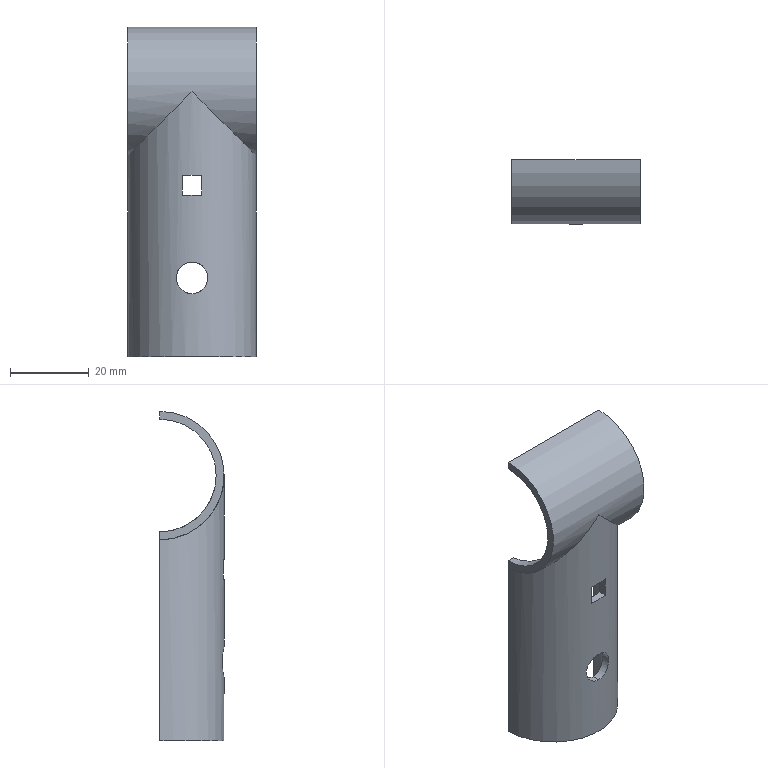Part | STEP file | F-D | 1 solid | 16 faces | box 32.6 x 16.3 x 83.6 mm | volume 7578 mm3 | plane 10 | cylinder 6 | commonest cylinder face diameters 8 x2 28.6 x2 32.6 x2
STEP:
#1=CARTESIAN_POINT('',(0.,48.7,-51.3));
#2=VERTEX_POINT('',#1);
#3=CARTESIAN_POINT('',(0.,48.7,-43.3));
#4=VERTEX_POINT('',#3);
#5=CARTESIAN_POINT('',(0.,48.7,-51.3));
#6=CARTESIAN_POINT('',(0.2485,48.7,-51.3));
#7=CARTESIAN_POINT('',(0.504,48.706,-51.277));
#8=CARTESIAN_POINT('',(0.8903,48.724,-51.202));
#9=CARTESIAN_POINT('',(1.02,48.732,-51.17));
#10=CARTESIAN_POINT('',(1.213,48.745,-51.112));
#11=CARTESIAN_POINT('',(1.31,48.753,-51.081));
#12=CARTESIAN_POINT('',(1.422,48.762,-51.039));
#13=CARTESIAN_POINT('',(1.478,48.767,-51.017));
#14=CARTESIAN_POINT('',(1.502,48.769,-51.007));
#15=CARTESIAN_POINT('',(1.518,48.771,-51.001));
#16=CARTESIAN_POINT('',(1.527,48.772,-50.997));
#17=CARTESIAN_POINT('',(1.643,48.783,-50.949));
#18=CARTESIAN_POINT('',(1.757,48.795,-50.896));
#19=CARTESIAN_POINT('',(1.932,48.815,-50.803));
#20=CARTESIAN_POINT('',(1.992,48.822,-50.769));
#21=CARTESIAN_POINT('',(2.082,48.834,-50.716));
#22=CARTESIAN_POINT('',(2.127,48.839,-50.688));
#23=CARTESIAN_POINT('',(2.18,48.847,-50.654));
#24=CARTESIAN_POINT('',(2.207,48.85,-50.636));
#25=CARTESIAN_POINT('',(2.218,48.852,-50.628));
#26=CARTESIAN_POINT('',(2.226,48.853,-50.623));
#27=CARTESIAN_POINT('',(2.231,48.854,-50.62));
#28=CARTESIAN_POINT('',(2.31,48.864,-50.567));
#29=CARTESIAN_POINT('',(2.4,48.878,-50.503));
#30=CARTESIAN_POINT('',(2.551,48.901,-50.382));
#31=CARTESIAN_POINT('',(2.604,48.909,-50.338));
#32=CARTESIAN_POINT('',(2.686,48.923,-50.264));
#33=CARTESIAN_POINT('',(2.714,48.928,-50.239));
#34=CARTESIAN_POINT('',(2.771,48.937,-50.185));
#35=CARTESIAN_POINT('',(2.798,48.942,-50.159));
#36=CARTESIAN_POINT('',(2.951,48.969,-50.006));
#37=CARTESIAN_POINT('',(3.05,48.987,-49.892));
#38=CARTESIAN_POINT('',(3.17,49.011,-49.741));
#39=CARTESIAN_POINT('',(3.205,49.018,-49.694));
#40=CARTESIAN_POINT('',(3.252,49.028,-49.629));
#41=CARTESIAN_POINT('',(3.274,49.032,-49.598));
#42=CARTESIAN_POINT('',(3.297,49.037,-49.565));
#43=CARTESIAN_POINT('',(3.308,49.039,-49.549));
#44=CARTESIAN_POINT('',(3.312,49.04,-49.542));
#45=CARTESIAN_POINT('',(3.315,49.041,-49.538));
#46=CARTESIAN_POINT('',(3.316,49.041,-49.537));
#47=CARTESIAN_POINT('',(3.401,49.058,-49.411));
#48=CARTESIAN_POINT('',(3.473,49.074,-49.29));
#49=CARTESIAN_POINT('',(3.566,49.095,-49.114));
#50=CARTESIAN_POINT('',(3.594,49.101,-49.056));
#51=CARTESIAN_POINT('',(3.634,49.11,-48.971));
#52=CARTESIAN_POINT('',(3.653,49.115,-48.929));
#53=CARTESIAN_POINT('',(3.674,49.12,-48.881));
#54=CARTESIAN_POINT('',(3.683,49.122,-48.861));
#55=CARTESIAN_POINT('',(3.689,49.123,-48.847));
#56=CARTESIAN_POINT('',(3.691,49.123,-48.842));
#57=CARTESIAN_POINT('',(3.907,49.174,-48.321));
#58=CARTESIAN_POINT('',(4.,49.198,-47.794));
#59=CARTESIAN_POINT('',(4.,49.198,-47.053));
#60=CARTESIAN_POINT('',(3.977,49.192,-46.798));
#61=CARTESIAN_POINT('',(3.902,49.174,-46.412));
#62=CARTESIAN_POINT('',(3.871,49.166,-46.282));
#63=CARTESIAN_POINT('',(3.813,49.152,-46.088));
#64=CARTESIAN_POINT('',(3.781,49.144,-45.991));
#65=CARTESIAN_POINT('',(3.739,49.135,-45.879));
#66=CARTESIAN_POINT('',(3.717,49.13,-45.823));
#67=CARTESIAN_POINT('',(3.708,49.127,-45.799));
#68=CARTESIAN_POINT('',(3.701,49.126,-45.783));
#69=CARTESIAN_POINT('',(3.697,49.125,-45.773));
#70=CARTESIAN_POINT('',(3.649,49.114,-45.658));
#71=CARTESIAN_POINT('',(3.597,49.102,-45.545));
#72=CARTESIAN_POINT('',(3.504,49.081,-45.369));
#73=CARTESIAN_POINT('',(3.47,49.074,-45.309));
#74=CARTESIAN_POINT('',(3.416,49.062,-45.219));
#75=CARTESIAN_POINT('',(3.388,49.056,-45.174));
#76=CARTESIAN_POINT('',(3.354,49.049,-45.12));
#77=CARTESIAN_POINT('',(3.336,49.045,-45.093));
#78=CARTESIAN_POINT('',(3.329,49.043,-45.082));
#79=CARTESIAN_POINT('',(3.324,49.042,-45.074));
#80=CARTESIAN_POINT('',(3.32,49.042,-45.069));
#81=CARTESIAN_POINT('',(3.271,49.032,-44.997));
#82=CARTESIAN_POINT('',(3.21,49.019,-44.91));
#83=CARTESIAN_POINT('',(3.09,48.995,-44.759));
#84=CARTESIAN_POINT('',(3.045,48.987,-44.705));
#85=CARTESIAN_POINT('',(2.97,48.973,-44.62));
#86=CARTESIAN_POINT('',(2.944,48.968,-44.591));
#87=CARTESIAN_POINT('',(2.888,48.958,-44.532));
#88=CARTESIAN_POINT('',(2.858,48.952,-44.501));
#89=CARTESIAN_POINT('',(2.712,48.927,-44.355));
#90=CARTESIAN_POINT('',(2.601,48.909,-44.258));
#91=CARTESIAN_POINT('',(2.45,48.885,-44.138));
#92=CARTESIAN_POINT('',(2.403,48.878,-44.102));
#93=CARTESIAN_POINT('',(2.336,48.868,-44.053));
#94=CARTESIAN_POINT('',(2.303,48.864,-44.03));
#95=CARTESIAN_POINT('',(2.268,48.859,-44.005));
#96=CARTESIAN_POINT('',(2.251,48.856,-43.993));
#97=CARTESIAN_POINT('',(2.243,48.855,-43.988));
#98=CARTESIAN_POINT('',(2.238,48.855,-43.985));
#99=CARTESIAN_POINT('',(2.237,48.854,-43.984));
#100=CARTESIAN_POINT('',(2.112,48.837,-43.9));
#101=CARTESIAN_POINT('',(1.991,48.822,-43.828));
#102=CARTESIAN_POINT('',(1.815,48.801,-43.735));
#103=CARTESIAN_POINT('',(1.758,48.795,-43.706));
#104=CARTESIAN_POINT('',(1.672,48.786,-43.666));
#105=CARTESIAN_POINT('',(1.63,48.782,-43.647));
#106=CARTESIAN_POINT('',(1.582,48.777,-43.626));
#107=CARTESIAN_POINT('',(1.561,48.775,-43.617));
#108=CARTESIAN_POINT('',(1.547,48.774,-43.611));
#109=CARTESIAN_POINT('',(1.542,48.773,-43.609));
#110=CARTESIAN_POINT('',(1.024,48.724,-43.394));
#111=CARTESIAN_POINT('',(0.497,48.7,-43.3));
#112=CARTESIAN_POINT('',(0.,48.7,-43.3));
#113=B_SPLINE_CURVE_WITH_KNOTS('',3,(#5,#6,#7,#8,#9,#10,#11,#12,#13,#14,#15,#16,#17,#18,#19,#20,#21,#22,#23,#24,#25,#26,#27,#28,#29,#30,#31,#32,#33,#34,#35,#36,#37,#38,#39,#40,#41,#42,#43,#44,#45,#46,#47,#48,#49,#50,#51,#52,#53,#54,#55,#56,#57,#58,#59,#60,#61,#62,#63,#64,#65,#66,#67,#68,#69,#70,#71,#72,#73,#74,#75,#76,#77,#78,#79,#80,#81,#82,#83,#84,#85,#86,#87,#88,#89,#90,#91,#92,#93,#94,#95,#96,#97,#98,#99,#100,#101,#102,#103,#104,#105,#106,#107,#108,#109,#110,#111,#112),.UNSPECIFIED.,.F.,.F.,(4,2,2,1,1,1,2,2,2,2,1,1,1,2,2,2,2,2,2,2,2,1,1,1,2,2,2,2,1,1,2,2,2,2,2,1,1,1,2,2,2,2,1,1,1,2,2,2,2,2,2,2,2,1,1,1,2,2,2,2,1,1,2,2,4),(0.5,0.5312,0.5469,0.5547,0.5586,0.5605,0.5615,0.5625,0.5781,0.5859,0.5898,0.5918,0.5928,0.5933,0.5937,0.6094,0.6172,0.6211,0.625,0.6406,0.6484,0.6523,0.6543,0.6553,0.6558,0.6562,0.6719,0.6797,0.6836,0.6855,0.6865,0.6875,0.75,0.7812,0.7969,0.8047,0.8086,0.8105,0.8115,0.8125,0.8281,0.8359,0.8398,0.8418,0.8428,0.8433,0.8437,0.8594,0.8672,0.8711,0.875,0.8906,0.8984,0.9023,0.9043,0.9053,0.9058,0.9062,0.9219,0.9297,0.9336,0.9355,0.9365,0.9375,1.),.UNSPECIFIED.);
#114=EDGE_CURVE('',#2,#4,#113,.T.);
#115=ORIENTED_EDGE('',*,*,#114,.T.);
#116=CARTESIAN_POINT('',(0.,50.7,-43.3));
#117=VERTEX_POINT('',#116);
#118=CARTESIAN_POINT('',(0.,130.,-43.3));
#119=DIRECTION('',(0.,1.,0.));
#120=VECTOR('',#119,1000.);
#121=LINE('',#118,#120);
#122=EDGE_CURVE('',#4,#117,#121,.T.);
#123=ORIENTED_EDGE('',*,*,#122,.T.);
#124=CARTESIAN_POINT('',(0.,50.7,-51.3));
#125=VERTEX_POINT('',#124);
#126=CARTESIAN_POINT('',(0.,50.7,-51.3));
#127=CARTESIAN_POINT('',(0.2655,50.7,-51.3));
#128=CARTESIAN_POINT('',(0.5263,50.707,-51.274));
#129=CARTESIAN_POINT('',(1.038,50.735,-51.172));
#130=CARTESIAN_POINT('',(1.29,50.756,-51.095));
#131=CARTESIAN_POINT('',(1.779,50.809,-50.892));
#132=CARTESIAN_POINT('',(2.009,50.84,-50.769));
#133=CARTESIAN_POINT('',(2.44,50.908,-50.481));
#134=CARTESIAN_POINT('',(2.641,50.945,-50.316));
#135=CARTESIAN_POINT('',(3.017,51.02,-49.94));
#136=CARTESIAN_POINT('',(3.182,51.058,-49.739));
#137=CARTESIAN_POINT('',(3.398,51.11,-49.415));
#138=CARTESIAN_POINT('',(3.465,51.126,-49.304));
#139=CARTESIAN_POINT('',(3.588,51.157,-49.074));
#140=CARTESIAN_POINT('',(3.643,51.172,-48.957));
#141=CARTESIAN_POINT('',(3.899,51.24,-48.342));
#142=CARTESIAN_POINT('',(4.,51.271,-47.83));
#143=CARTESIAN_POINT('',(4.,51.271,-47.035));
#144=CARTESIAN_POINT('',(3.975,51.263,-46.775));
#145=CARTESIAN_POINT('',(3.898,51.242,-46.391));
#146=CARTESIAN_POINT('',(3.866,51.233,-46.264));
#147=CARTESIAN_POINT('',(3.79,51.211,-46.013));
#148=CARTESIAN_POINT('',(3.745,51.199,-45.887));
#149=CARTESIAN_POINT('',(3.593,51.158,-45.522));
#150=CARTESIAN_POINT('',(3.471,51.127,-45.293));
#151=CARTESIAN_POINT('',(3.182,51.058,-44.862));
#152=CARTESIAN_POINT('',(3.016,51.02,-44.659));
#153=CARTESIAN_POINT('',(2.642,50.945,-44.285));
#154=CARTESIAN_POINT('',(2.44,50.908,-44.119));
#155=CARTESIAN_POINT('',(2.009,50.84,-43.831));
#156=CARTESIAN_POINT('',(1.78,50.809,-43.708));
#157=CARTESIAN_POINT('',(1.043,50.73,-43.402));
#158=CARTESIAN_POINT('',(0.5311,50.7,-43.3));
#159=CARTESIAN_POINT('',(0.,50.7,-43.3));
#160=B_SPLINE_CURVE_WITH_KNOTS('',3,(#126,#127,#128,#129,#130,#131,#132,#133,#134,#135,#136,#137,#138,#139,#140,#141,#142,#143,#144,#145,#146,#147,#148,#149,#150,#151,#152,#153,#154,#155,#156,#157,#158,#159),.UNSPECIFIED.,.F.,.F.,(4,2,2,2,2,2,2,2,2,2,2,2,2,2,2,2,4),(0.,0.0625,0.125,0.1875,0.25,0.3125,0.3438,0.375,0.5,0.5625,0.5938,0.625,0.6875,0.75,0.8125,0.875,1.),.UNSPECIFIED.);
#161=EDGE_CURVE('',#125,#117,#160,.T.);
#162=ORIENTED_EDGE('',*,*,#161,.F.);
#163=CARTESIAN_POINT('',(0.,130.,-51.3));
#164=DIRECTION('',(0.,1.,0.));
#165=VECTOR('',#164,1000.);
#166=LINE('',#163,#165);
#167=EDGE_CURVE('',#2,#125,#166,.T.);
#168=ORIENTED_EDGE('',*,*,#167,.F.);
#169=EDGE_LOOP('',(#115,#123,#162,#168));
#170=FACE_OUTER_BOUND('',#169,.T.);
#171=CARTESIAN_POINT('',(0.,130.,-47.3));
#172=DIRECTION('',(0.,1.,0.));
#173=DIRECTION('',(0.,0.,-1.));
#174=AXIS2_PLACEMENT_3D('',#171,#172,#173);
#175=CYLINDRICAL_SURFACE('',#174,4.);
#176=ADVANCED_FACE('',(#170),#175,.F.);
#177=CARTESIAN_POINT('',(16.3,65.,-16.3));
#178=VERTEX_POINT('',#177);
#179=CARTESIAN_POINT('',(16.3,65.,16.3));
#180=VERTEX_POINT('',#179);
#181=CARTESIAN_POINT('',(16.3,65.,0.));
#182=DIRECTION('',(-1.,0.,0.));
#183=DIRECTION('',(0.,0.,1.));
#184=AXIS2_PLACEMENT_3D('',#181,#182,#183);
#185=CIRCLE('',#184,16.3);
#186=EDGE_CURVE('',#178,#180,#185,.T.);
#187=ORIENTED_EDGE('',*,*,#186,.T.);
#188=CARTESIAN_POINT('',(-16.3,65.,16.3));
#189=VERTEX_POINT('',#188);
#190=CARTESIAN_POINT('',(16.3,65.,16.3));
#191=DIRECTION('',(1.,0.,0.));
#192=VECTOR('',#191,1000.);
#193=LINE('',#190,#192);
#194=EDGE_CURVE('',#189,#180,#193,.T.);
#195=ORIENTED_EDGE('',*,*,#194,.F.);
#196=CARTESIAN_POINT('',(-16.3,65.,-16.3));
#197=VERTEX_POINT('',#196);
#198=CARTESIAN_POINT('',(-16.3,65.,0.));
#199=DIRECTION('',(1.,0.,0.));
#200=DIRECTION('',(0.,1.,0.));
#201=AXIS2_PLACEMENT_3D('',#198,#199,#200);
#202=CIRCLE('',#201,16.3);
#203=EDGE_CURVE('',#189,#197,#202,.T.);
#204=ORIENTED_EDGE('',*,*,#203,.T.);
#205=CARTESIAN_POINT('',(0.,48.7,0.));
#206=VERTEX_POINT('',#205);
#207=CARTESIAN_POINT('',(0.,48.7,0.));
#208=CARTESIAN_POINT('',(-9.548,48.7,-9.548));
#209=CARTESIAN_POINT('',(-16.3,55.452,-16.3));
#210=CARTESIAN_POINT('',(-16.3,65.,-16.3));
#211=(BOUNDED_CURVE()B_SPLINE_CURVE(3,(#207,#208,#209,#210),.UNSPECIFIED.,.F.,.F.)B_SPLINE_CURVE_WITH_KNOTS((4,4),(4.712,6.283),.UNSPECIFIED.)CURVE()GEOMETRIC_REPRESENTATION_ITEM()RATIONAL_B_SPLINE_CURVE((1.,0.8047,0.8047,1.))REPRESENTATION_ITEM(''));
#212=EDGE_CURVE('',#206,#197,#211,.T.);
#213=ORIENTED_EDGE('',*,*,#212,.F.);
#214=CARTESIAN_POINT('',(16.3,65.,-16.3));
#215=CARTESIAN_POINT('',(16.3,55.452,-16.3));
#216=CARTESIAN_POINT('',(9.548,48.7,-9.548));
#217=CARTESIAN_POINT('',(0.,48.7,0.));
#218=(BOUNDED_CURVE()B_SPLINE_CURVE(3,(#214,#215,#216,#217),.UNSPECIFIED.,.F.,.F.)B_SPLINE_CURVE_WITH_KNOTS((4,4),(3.142,4.712),.UNSPECIFIED.)CURVE()GEOMETRIC_REPRESENTATION_ITEM()RATIONAL_B_SPLINE_CURVE((1.,0.8047,0.8047,1.))REPRESENTATION_ITEM(''));
#219=EDGE_CURVE('',#178,#206,#218,.T.);
#220=ORIENTED_EDGE('',*,*,#219,.F.);
#221=EDGE_LOOP('',(#187,#195,#204,#213,#220));
#222=FACE_OUTER_BOUND('',#221,.T.);
#223=CARTESIAN_POINT('',(16.3,65.,0.));
#224=DIRECTION('',(1.,0.,0.));
#225=DIRECTION('',(0.,0.,1.));
#226=AXIS2_PLACEMENT_3D('',#223,#224,#225);
#227=CYLINDRICAL_SURFACE('',#226,16.3);
#228=ADVANCED_FACE('',(#222),#227,.T.);
#229=ORIENTED_EDGE('',*,*,#203,.F.);
#230=CARTESIAN_POINT('',(-16.3,65.,14.3));
#231=VERTEX_POINT('',#230);
#232=CARTESIAN_POINT('',(-16.3,65.,0.));
#233=DIRECTION('',(0.,0.,-1.));
#234=VECTOR('',#233,1000.);
#235=LINE('',#232,#234);
#236=EDGE_CURVE('',#189,#231,#235,.T.);
#237=ORIENTED_EDGE('',*,*,#236,.T.);
#238=CARTESIAN_POINT('',(-16.3,65.,-14.3));
#239=VERTEX_POINT('',#238);
#240=CARTESIAN_POINT('',(-16.3,65.,0.));
#241=DIRECTION('',(-1.,0.,0.));
#242=DIRECTION('',(0.,-1.,0.));
#243=AXIS2_PLACEMENT_3D('',#240,#241,#242);
#244=CIRCLE('',#243,14.3);
#245=EDGE_CURVE('',#239,#231,#244,.T.);
#246=ORIENTED_EDGE('',*,*,#245,.F.);
#247=CARTESIAN_POINT('',(-16.3,65.,-16.3));
#248=DIRECTION('',(0.,0.,1.));
#249=VECTOR('',#248,1000.);
#250=LINE('',#247,#249);
#251=EDGE_CURVE('',#197,#239,#250,.T.);
#252=ORIENTED_EDGE('',*,*,#251,.F.);
#253=EDGE_LOOP('',(#229,#237,#246,#252));
#254=FACE_OUTER_BOUND('',#253,.T.);
#255=CARTESIAN_POINT('',(-16.3,65.,0.));
#256=DIRECTION('',(-1.,0.,0.));
#257=DIRECTION('',(0.,0.,1.));
#258=AXIS2_PLACEMENT_3D('',#255,#256,#257);
#259=PLANE('',#258);
#260=ADVANCED_FACE('',(#254),#259,.T.);
#261=CARTESIAN_POINT('',(-14.3,65.,-14.3));
#262=VERTEX_POINT('',#261);
#263=CARTESIAN_POINT('',(16.3,65.,-14.3));
#264=DIRECTION('',(-1.,0.,0.));
#265=VECTOR('',#264,1000.);
#266=LINE('',#263,#265);
#267=EDGE_CURVE('',#262,#239,#266,.T.);
#268=ORIENTED_EDGE('',*,*,#267,.F.);
#269=CARTESIAN_POINT('',(-14.3,65.,-67.3));
#270=VERTEX_POINT('',#269);
#271=CARTESIAN_POINT('',(-14.3,65.,-76.464));
#272=DIRECTION('',(0.,0.,1.));
#273=VECTOR('',#272,1000.);
#274=LINE('',#271,#273);
#275=EDGE_CURVE('',#270,#262,#274,.T.);
#276=ORIENTED_EDGE('',*,*,#275,.F.);
#277=CARTESIAN_POINT('',(-16.3,65.,-67.3));
#278=VERTEX_POINT('',#277);
#279=CARTESIAN_POINT('',(-26.203,65.,-67.3));
#280=DIRECTION('',(1.,0.,0.));
#281=VECTOR('',#280,1000.);
#282=LINE('',#279,#281);
#283=EDGE_CURVE('',#278,#270,#282,.T.);
#284=ORIENTED_EDGE('',*,*,#283,.F.);
#285=CARTESIAN_POINT('',(-16.3,65.,0.));
#286=DIRECTION('',(0.,0.,-1.));
#287=VECTOR('',#286,1000.);
#288=LINE('',#285,#287);
#289=EDGE_CURVE('',#197,#278,#288,.T.);
#290=ORIENTED_EDGE('',*,*,#289,.F.);
#291=ORIENTED_EDGE('',*,*,#251,.T.);
#292=EDGE_LOOP('',(#268,#276,#284,#290,#291));
#293=FACE_OUTER_BOUND('',#292,.T.);
#294=CARTESIAN_POINT('',(16.3,65.,-16.3));
#295=DIRECTION('',(0.,-1.,0.));
#296=DIRECTION('',(-1.,0.,0.));
#297=AXIS2_PLACEMENT_3D('',#294,#295,#296);
#298=PLANE('',#297);
#299=ADVANCED_FACE('',(#293),#298,.F.);
#300=ORIENTED_EDGE('',*,*,#114,.F.);
#301=CARTESIAN_POINT('',(0.,48.7,-43.3));
#302=CARTESIAN_POINT('',(-0.2485,48.7,-43.3));
#303=CARTESIAN_POINT('',(-0.504,48.706,-43.323));
#304=CARTESIAN_POINT('',(-0.8903,48.724,-43.398));
#305=CARTESIAN_POINT('',(-1.02,48.732,-43.43));
#306=CARTESIAN_POINT('',(-1.213,48.745,-43.488));
#307=CARTESIAN_POINT('',(-1.31,48.753,-43.519));
#308=CARTESIAN_POINT('',(-1.422,48.762,-43.561));
#309=CARTESIAN_POINT('',(-1.478,48.767,-43.583));
#310=CARTESIAN_POINT('',(-1.502,48.769,-43.593));
#311=CARTESIAN_POINT('',(-1.518,48.771,-43.599));
#312=CARTESIAN_POINT('',(-1.527,48.772,-43.603));
#313=CARTESIAN_POINT('',(-1.643,48.783,-43.651));
#314=CARTESIAN_POINT('',(-1.757,48.795,-43.704));
#315=CARTESIAN_POINT('',(-1.932,48.815,-43.797));
#316=CARTESIAN_POINT('',(-1.992,48.822,-43.831));
#317=CARTESIAN_POINT('',(-2.082,48.834,-43.884));
#318=CARTESIAN_POINT('',(-2.127,48.839,-43.912));
#319=CARTESIAN_POINT('',(-2.18,48.847,-43.946));
#320=CARTESIAN_POINT('',(-2.207,48.85,-43.964));
#321=CARTESIAN_POINT('',(-2.218,48.852,-43.972));
#322=CARTESIAN_POINT('',(-2.226,48.853,-43.977));
#323=CARTESIAN_POINT('',(-2.231,48.854,-43.98));
#324=CARTESIAN_POINT('',(-2.31,48.864,-44.033));
#325=CARTESIAN_POINT('',(-2.4,48.878,-44.097));
#326=CARTESIAN_POINT('',(-2.551,48.901,-44.218));
#327=CARTESIAN_POINT('',(-2.604,48.909,-44.262));
#328=CARTESIAN_POINT('',(-2.686,48.923,-44.336));
#329=CARTESIAN_POINT('',(-2.714,48.928,-44.361));
#330=CARTESIAN_POINT('',(-2.771,48.937,-44.415));
#331=CARTESIAN_POINT('',(-2.798,48.942,-44.441));
#332=CARTESIAN_POINT('',(-2.951,48.969,-44.594));
#333=CARTESIAN_POINT('',(-3.05,48.987,-44.708));
#334=CARTESIAN_POINT('',(-3.17,49.011,-44.859));
#335=CARTESIAN_POINT('',(-3.205,49.018,-44.906));
#336=CARTESIAN_POINT('',(-3.252,49.028,-44.971));
#337=CARTESIAN_POINT('',(-3.274,49.032,-45.002));
#338=CARTESIAN_POINT('',(-3.297,49.037,-45.035));
#339=CARTESIAN_POINT('',(-3.308,49.039,-45.051));
#340=CARTESIAN_POINT('',(-3.312,49.04,-45.058));
#341=CARTESIAN_POINT('',(-3.315,49.041,-45.062));
#342=CARTESIAN_POINT('',(-3.316,49.041,-45.063));
#343=CARTESIAN_POINT('',(-3.401,49.058,-45.189));
#344=CARTESIAN_POINT('',(-3.473,49.074,-45.31));
#345=CARTESIAN_POINT('',(-3.566,49.095,-45.486));
#346=CARTESIAN_POINT('',(-3.594,49.101,-45.544));
#347=CARTESIAN_POINT('',(-3.634,49.11,-45.629));
#348=CARTESIAN_POINT('',(-3.653,49.115,-45.671));
#349=CARTESIAN_POINT('',(-3.674,49.12,-45.719));
#350=CARTESIAN_POINT('',(-3.683,49.122,-45.739));
#351=CARTESIAN_POINT('',(-3.689,49.123,-45.753));
#352=CARTESIAN_POINT('',(-3.691,49.123,-45.758));
#353=CARTESIAN_POINT('',(-3.907,49.174,-46.279));
#354=CARTESIAN_POINT('',(-4.,49.198,-46.806));
#355=CARTESIAN_POINT('',(-4.,49.198,-47.547));
#356=CARTESIAN_POINT('',(-3.977,49.192,-47.802));
#357=CARTESIAN_POINT('',(-3.902,49.174,-48.188));
#358=CARTESIAN_POINT('',(-3.871,49.166,-48.318));
#359=CARTESIAN_POINT('',(-3.813,49.152,-48.512));
#360=CARTESIAN_POINT('',(-3.781,49.144,-48.609));
#361=CARTESIAN_POINT('',(-3.739,49.135,-48.721));
#362=CARTESIAN_POINT('',(-3.717,49.13,-48.777));
#363=CARTESIAN_POINT('',(-3.708,49.127,-48.801));
#364=CARTESIAN_POINT('',(-3.701,49.126,-48.817));
#365=CARTESIAN_POINT('',(-3.697,49.125,-48.827));
#366=CARTESIAN_POINT('',(-3.649,49.114,-48.942));
#367=CARTESIAN_POINT('',(-3.597,49.102,-49.055));
#368=CARTESIAN_POINT('',(-3.504,49.081,-49.231));
#369=CARTESIAN_POINT('',(-3.47,49.074,-49.291));
#370=CARTESIAN_POINT('',(-3.416,49.062,-49.381));
#371=CARTESIAN_POINT('',(-3.388,49.056,-49.426));
#372=CARTESIAN_POINT('',(-3.354,49.049,-49.48));
#373=CARTESIAN_POINT('',(-3.336,49.045,-49.507));
#374=CARTESIAN_POINT('',(-3.329,49.043,-49.518));
#375=CARTESIAN_POINT('',(-3.324,49.042,-49.526));
#376=CARTESIAN_POINT('',(-3.32,49.042,-49.531));
#377=CARTESIAN_POINT('',(-3.271,49.032,-49.603));
#378=CARTESIAN_POINT('',(-3.21,49.019,-49.69));
#379=CARTESIAN_POINT('',(-3.09,48.995,-49.841));
#380=CARTESIAN_POINT('',(-3.045,48.987,-49.895));
#381=CARTESIAN_POINT('',(-2.97,48.973,-49.98));
#382=CARTESIAN_POINT('',(-2.944,48.968,-50.009));
#383=CARTESIAN_POINT('',(-2.888,48.958,-50.068));
#384=CARTESIAN_POINT('',(-2.858,48.952,-50.099));
#385=CARTESIAN_POINT('',(-2.712,48.927,-50.245));
#386=CARTESIAN_POINT('',(-2.601,48.909,-50.342));
#387=CARTESIAN_POINT('',(-2.45,48.885,-50.462));
#388=CARTESIAN_POINT('',(-2.403,48.878,-50.498));
#389=CARTESIAN_POINT('',(-2.336,48.868,-50.547));
#390=CARTESIAN_POINT('',(-2.303,48.864,-50.57));
#391=CARTESIAN_POINT('',(-2.268,48.859,-50.595));
#392=CARTESIAN_POINT('',(-2.251,48.856,-50.607));
#393=CARTESIAN_POINT('',(-2.243,48.855,-50.612));
#394=CARTESIAN_POINT('',(-2.238,48.855,-50.615));
#395=CARTESIAN_POINT('',(-2.237,48.854,-50.616));
#396=CARTESIAN_POINT('',(-2.112,48.837,-50.7));
#397=CARTESIAN_POINT('',(-1.991,48.822,-50.772));
#398=CARTESIAN_POINT('',(-1.815,48.801,-50.865));
#399=CARTESIAN_POINT('',(-1.758,48.795,-50.894));
#400=CARTESIAN_POINT('',(-1.672,48.786,-50.934));
#401=CARTESIAN_POINT('',(-1.63,48.782,-50.953));
#402=CARTESIAN_POINT('',(-1.582,48.777,-50.974));
#403=CARTESIAN_POINT('',(-1.561,48.775,-50.983));
#404=CARTESIAN_POINT('',(-1.547,48.774,-50.989));
#405=CARTESIAN_POINT('',(-1.542,48.773,-50.991));
#406=CARTESIAN_POINT('',(-1.024,48.724,-51.206));
#407=CARTESIAN_POINT('',(-0.497,48.7,-51.3));
#408=CARTESIAN_POINT('',(0.,48.7,-51.3));
#409=B_SPLINE_CURVE_WITH_KNOTS('',3,(#301,#302,#303,#304,#305,#306,#307,#308,#309,#310,#311,#312,#313,#314,#315,#316,#317,#318,#319,#320,#321,#322,#323,#324,#325,#326,#327,#328,#329,#330,#331,#332,#333,#334,#335,#336,#337,#338,#339,#340,#341,#342,#343,#344,#345,#346,#347,#348,#349,#350,#351,#352,#353,#354,#355,#356,#357,#358,#359,#360,#361,#362,#363,#364,#365,#366,#367,#368,#369,#370,#371,#372,#373,#374,#375,#376,#377,#378,#379,#380,#381,#382,#383,#384,#385,#386,#387,#388,#389,#390,#391,#392,#393,#394,#395,#396,#397,#398,#399,#400,#401,#402,#403,#404,#405,#406,#407,#408),.UNSPECIFIED.,.F.,.F.,(4,2,2,1,1,1,2,2,2,2,1,1,1,2,2,2,2,2,2,2,2,1,1,1,2,2,2,2,1,1,2,2,2,2,2,1,1,1,2,2,2,2,1,1,1,2,2,2,2,2,2,2,2,1,1,1,2,2,2,2,1,1,2,2,4),(0.,0.03125,0.04687,0.05469,0.05859,0.06055,0.06152,0.0625,0.07812,0.08594,0.08984,0.0918,0.09277,0.09326,0.09375,0.1094,0.1172,0.1211,0.125,0.1406,0.1484,0.1523,0.1543,0.1553,0.1558,0.1562,0.1719,0.1797,0.1836,0.1855,0.1865,0.1875,0.25,0.2812,0.2969,0.3047,0.3086,0.3105,0.3115,0.3125,0.3281,0.3359,0.3398,0.3418,0.3428,0.3433,0.3437,0.3594,0.3672,0.3711,0.375,0.3906,0.3984,0.4023,0.4043,0.4053,0.4058,0.4062,0.4219,0.4297,0.4336,0.4355,0.4365,0.4375,0.5),.UNSPECIFIED.);
#410=EDGE_CURVE('',#4,#2,#409,.T.);
#411=ORIENTED_EDGE('',*,*,#410,.F.);
#412=EDGE_LOOP('',(#300,#411));
#413=FACE_BOUND('',#412,.T.);
#414=CARTESIAN_POINT('',(-2.5,48.893,-21.3));
#415=VERTEX_POINT('',#414);
#416=CARTESIAN_POINT('',(2.5,48.893,-21.3));
#417=VERTEX_POINT('',#416);
#418=CARTESIAN_POINT('',(0.,65.,-21.3));
#419=DIRECTION('',(0.,0.,1.));
#420=DIRECTION('',(1.,0.,0.));
#421=AXIS2_PLACEMENT_3D('',#418,#419,#420);
#422=CIRCLE('',#421,16.3);
#423=EDGE_CURVE('',#415,#417,#422,.T.);
#424=ORIENTED_EDGE('',*,*,#423,.T.);
#425=CARTESIAN_POINT('',(2.5,48.893,-26.3));
#426=VERTEX_POINT('',#425);
#427=CARTESIAN_POINT('',(2.5,48.893,-76.464));
#428=DIRECTION('',(0.,0.,-1.));
#429=VECTOR('',#428,1000.);
#430=LINE('',#427,#429);
#431=EDGE_CURVE('',#417,#426,#430,.T.);
#432=ORIENTED_EDGE('',*,*,#431,.T.);
#433=CARTESIAN_POINT('',(-2.5,48.893,-26.3));
#434=VERTEX_POINT('',#433);
#435=CARTESIAN_POINT('',(0.,65.,-26.3));
#436=DIRECTION('',(0.,0.,-1.));
#437=DIRECTION('',(-1.,0.,0.));
#438=AXIS2_PLACEMENT_3D('',#435,#436,#437);
#439=CIRCLE('',#438,16.3);
#440=EDGE_CURVE('',#426,#434,#439,.T.);
#441=ORIENTED_EDGE('',*,*,#440,.T.);
#442=CARTESIAN_POINT('',(-2.5,48.893,-76.464));
#443=DIRECTION('',(0.,0.,1.));
#444=VECTOR('',#443,1000.);
#445=LINE('',#442,#444);
#446=EDGE_CURVE('',#434,#415,#445,.T.);
#447=ORIENTED_EDGE('',*,*,#446,.T.);
#448=EDGE_LOOP('',(#424,#432,#441,#447));
#449=FACE_BOUND('',#448,.T.);
#450=CARTESIAN_POINT('',(16.3,65.,-67.3));
#451=VERTEX_POINT('',#450);
#452=CARTESIAN_POINT('',(16.3,65.,-76.464));
#453=DIRECTION('',(0.,0.,-1.));
#454=VECTOR('',#453,1000.);
#455=LINE('',#452,#454);
#456=EDGE_CURVE('',#178,#451,#455,.T.);
#457=ORIENTED_EDGE('',*,*,#456,.F.);
#458=ORIENTED_EDGE('',*,*,#219,.T.);
#459=ORIENTED_EDGE('',*,*,#212,.T.);
#460=ORIENTED_EDGE('',*,*,#289,.T.);
#461=CARTESIAN_POINT('',(0.,65.,-67.3));
#462=DIRECTION('',(0.,0.,-1.));
#463=DIRECTION('',(-1.,0.,0.));
#464=AXIS2_PLACEMENT_3D('',#461,#462,#463);
#465=CIRCLE('',#464,16.3);
#466=EDGE_CURVE('',#451,#278,#465,.T.);
#467=ORIENTED_EDGE('',*,*,#466,.F.);
#468=EDGE_LOOP('',(#457,#458,#459,#460,#467));
#469=FACE_OUTER_BOUND('',#468,.T.);
#470=CARTESIAN_POINT('',(0.,65.,-76.464));
#471=DIRECTION('',(0.,0.,-1.));
#472=DIRECTION('',(1.,0.,0.));
#473=AXIS2_PLACEMENT_3D('',#470,#471,#472);
#474=CYLINDRICAL_SURFACE('',#473,16.3);
#475=ADVANCED_FACE('',(#413,#449,#469),#474,.T.);
#476=ORIENTED_EDGE('',*,*,#161,.T.);
#477=CARTESIAN_POINT('',(0.,50.7,-43.3));
#478=CARTESIAN_POINT('',(-0.2655,50.7,-43.3));
#479=CARTESIAN_POINT('',(-0.5263,50.707,-43.326));
#480=CARTESIAN_POINT('',(-1.038,50.735,-43.428));
#481=CARTESIAN_POINT('',(-1.29,50.756,-43.505));
#482=CARTESIAN_POINT('',(-1.779,50.809,-43.708));
#483=CARTESIAN_POINT('',(-2.009,50.84,-43.831));
#484=CARTESIAN_POINT('',(-2.44,50.908,-44.119));
#485=CARTESIAN_POINT('',(-2.641,50.945,-44.284));
#486=CARTESIAN_POINT('',(-3.017,51.02,-44.66));
#487=CARTESIAN_POINT('',(-3.182,51.058,-44.861));
#488=CARTESIAN_POINT('',(-3.398,51.11,-45.185));
#489=CARTESIAN_POINT('',(-3.465,51.126,-45.296));
#490=CARTESIAN_POINT('',(-3.588,51.157,-45.526));
#491=CARTESIAN_POINT('',(-3.643,51.172,-45.643));
#492=CARTESIAN_POINT('',(-3.899,51.24,-46.258));
#493=CARTESIAN_POINT('',(-4.,51.271,-46.77));
#494=CARTESIAN_POINT('',(-4.,51.271,-47.565));
#495=CARTESIAN_POINT('',(-3.975,51.263,-47.825));
#496=CARTESIAN_POINT('',(-3.898,51.242,-48.209));
#497=CARTESIAN_POINT('',(-3.866,51.233,-48.336));
#498=CARTESIAN_POINT('',(-3.79,51.211,-48.587));
#499=CARTESIAN_POINT('',(-3.745,51.199,-48.713));
#500=CARTESIAN_POINT('',(-3.593,51.158,-49.078));
#501=CARTESIAN_POINT('',(-3.471,51.127,-49.307));
#502=CARTESIAN_POINT('',(-3.182,51.058,-49.738));
#503=CARTESIAN_POINT('',(-3.016,51.02,-49.941));
#504=CARTESIAN_POINT('',(-2.642,50.945,-50.315));
#505=CARTESIAN_POINT('',(-2.44,50.908,-50.481));
#506=CARTESIAN_POINT('',(-2.009,50.84,-50.769));
#507=CARTESIAN_POINT('',(-1.78,50.809,-50.892));
#508=CARTESIAN_POINT('',(-1.043,50.73,-51.198));
#509=CARTESIAN_POINT('',(-0.5311,50.7,-51.3));
#510=CARTESIAN_POINT('',(0.,50.7,-51.3));
#511=B_SPLINE_CURVE_WITH_KNOTS('',3,(#477,#478,#479,#480,#481,#482,#483,#484,#485,#486,#487,#488,#489,#490,#491,#492,#493,#494,#495,#496,#497,#498,#499,#500,#501,#502,#503,#504,#505,#506,#507,#508,#509,#510),.UNSPECIFIED.,.F.,.F.,(4,2,2,2,2,2,2,2,2,2,2,2,2,2,2,2,4),(0.,0.0625,0.125,0.1875,0.25,0.3125,0.3438,0.375,0.5,0.5625,0.5938,0.625,0.6875,0.75,0.8125,0.875,1.),.UNSPECIFIED.);
#512=EDGE_CURVE('',#117,#125,#511,.T.);
#513=ORIENTED_EDGE('',*,*,#512,.T.);
#514=EDGE_LOOP('',(#476,#513));
#515=FACE_BOUND('',#514,.T.);
#516=CARTESIAN_POINT('',(2.5,50.92,-21.3));
#517=VERTEX_POINT('',#516);
#518=CARTESIAN_POINT('',(2.5,50.92,-26.3));
#519=VERTEX_POINT('',#518);
#520=CARTESIAN_POINT('',(2.5,50.92,-76.464));
#521=DIRECTION('',(0.,0.,-1.));
#522=VECTOR('',#521,1000.);
#523=LINE('',#520,#522);
#524=EDGE_CURVE('',#517,#519,#523,.T.);
#525=ORIENTED_EDGE('',*,*,#524,.F.);
#526=CARTESIAN_POINT('',(-2.5,50.92,-21.3));
#527=VERTEX_POINT('',#526);
#528=CARTESIAN_POINT('',(0.,65.,-21.3));
#529=DIRECTION('',(0.,0.,1.));
#530=DIRECTION('',(1.,0.,0.));
#531=AXIS2_PLACEMENT_3D('',#528,#529,#530);
#532=CIRCLE('',#531,14.3);
#533=EDGE_CURVE('',#527,#517,#532,.T.);
#534=ORIENTED_EDGE('',*,*,#533,.F.);
#535=CARTESIAN_POINT('',(-2.5,50.92,-26.3));
#536=VERTEX_POINT('',#535);
#537=CARTESIAN_POINT('',(-2.5,50.92,-76.464));
#538=DIRECTION('',(0.,0.,1.));
#539=VECTOR('',#538,1000.);
#540=LINE('',#537,#539);
#541=EDGE_CURVE('',#536,#527,#540,.T.);
#542=ORIENTED_EDGE('',*,*,#541,.F.);
#543=CARTESIAN_POINT('',(0.,65.,-26.3));
#544=DIRECTION('',(0.,0.,-1.));
#545=DIRECTION('',(-1.,0.,0.));
#546=AXIS2_PLACEMENT_3D('',#543,#544,#545);
#547=CIRCLE('',#546,14.3);
#548=EDGE_CURVE('',#519,#536,#547,.T.);
#549=ORIENTED_EDGE('',*,*,#548,.F.);
#550=EDGE_LOOP('',(#525,#534,#542,#549));
#551=FACE_BOUND('',#550,.T.);
#552=CARTESIAN_POINT('',(14.3,65.,-67.3));
#553=VERTEX_POINT('',#552);
#554=CARTESIAN_POINT('',(0.,65.,-67.3));
#555=DIRECTION('',(0.,0.,-1.));
#556=DIRECTION('',(-1.,0.,0.));
#557=AXIS2_PLACEMENT_3D('',#554,#555,#556);
#558=CIRCLE('',#557,14.3);
#559=EDGE_CURVE('',#553,#270,#558,.T.);
#560=ORIENTED_EDGE('',*,*,#559,.T.);
#561=ORIENTED_EDGE('',*,*,#275,.T.);
#562=CARTESIAN_POINT('',(0.,50.7,0.));
#563=VERTEX_POINT('',#562);
#564=CARTESIAN_POINT('',(-14.3,65.,-14.3));
#565=CARTESIAN_POINT('',(-14.3,56.623,-14.3));
#566=CARTESIAN_POINT('',(-8.377,50.7,-8.377));
#567=CARTESIAN_POINT('',(0.,50.7,0.));
#568=(BOUNDED_CURVE()B_SPLINE_CURVE(3,(#564,#565,#566,#567),.UNSPECIFIED.,.F.,.F.)B_SPLINE_CURVE_WITH_KNOTS((4,4),(0.,1.571),.UNSPECIFIED.)CURVE()GEOMETRIC_REPRESENTATION_ITEM()RATIONAL_B_SPLINE_CURVE((1.,0.8047,0.8047,1.))REPRESENTATION_ITEM(''));
#569=EDGE_CURVE('',#262,#563,#568,.T.);
#570=ORIENTED_EDGE('',*,*,#569,.T.);
#571=CARTESIAN_POINT('',(14.3,65.,-14.3));
#572=VERTEX_POINT('',#571);
#573=CARTESIAN_POINT('',(0.,50.7,0.));
#574=CARTESIAN_POINT('',(8.377,50.7,-8.377));
#575=CARTESIAN_POINT('',(14.3,56.623,-14.3));
#576=CARTESIAN_POINT('',(14.3,65.,-14.3));
#577=(BOUNDED_CURVE()B_SPLINE_CURVE(3,(#573,#574,#575,#576),.UNSPECIFIED.,.F.,.F.)B_SPLINE_CURVE_WITH_KNOTS((4,4),(1.571,3.142),.UNSPECIFIED.)CURVE()GEOMETRIC_REPRESENTATION_ITEM()RATIONAL_B_SPLINE_CURVE((1.,0.8047,0.8047,1.))REPRESENTATION_ITEM(''));
#578=EDGE_CURVE('',#563,#572,#577,.T.);
#579=ORIENTED_EDGE('',*,*,#578,.T.);
#580=CARTESIAN_POINT('',(14.3,65.,-76.464));
#581=DIRECTION('',(0.,0.,-1.));
#582=VECTOR('',#581,1000.);
#583=LINE('',#580,#582);
#584=EDGE_CURVE('',#572,#553,#583,.T.);
#585=ORIENTED_EDGE('',*,*,#584,.T.);
#586=EDGE_LOOP('',(#560,#561,#570,#579,#585));
#587=FACE_OUTER_BOUND('',#586,.T.);
#588=CARTESIAN_POINT('',(0.,65.,-76.464));
#589=DIRECTION('',(0.,0.,-1.));
#590=DIRECTION('',(1.,0.,0.));
#591=AXIS2_PLACEMENT_3D('',#588,#589,#590);
#592=CYLINDRICAL_SURFACE('',#591,14.3);
#593=ADVANCED_FACE('',(#515,#551,#587),#592,.F.);
#594=ORIENTED_EDGE('',*,*,#466,.T.);
#595=ORIENTED_EDGE('',*,*,#283,.T.);
#596=ORIENTED_EDGE('',*,*,#559,.F.);
#597=CARTESIAN_POINT('',(-26.203,65.,-67.3));
#598=DIRECTION('',(1.,0.,0.));
#599=VECTOR('',#598,1000.);
#600=LINE('',#597,#599);
#601=EDGE_CURVE('',#553,#451,#600,.T.);
#602=ORIENTED_EDGE('',*,*,#601,.T.);
#603=EDGE_LOOP('',(#594,#595,#596,#602));
#604=FACE_OUTER_BOUND('',#603,.T.);
#605=CARTESIAN_POINT('',(-26.203,126.385,-67.3));
#606=DIRECTION('',(0.,0.,-1.));
#607=DIRECTION('',(0.,-1.,0.));
#608=AXIS2_PLACEMENT_3D('',#605,#606,#607);
#609=PLANE('',#608);
#610=ADVANCED_FACE('',(#604),#609,.T.);
#611=CARTESIAN_POINT('',(16.3,65.,14.3));
#612=VERTEX_POINT('',#611);
#613=CARTESIAN_POINT('',(16.3,65.,20.242));
#614=DIRECTION('',(0.,0.,-1.));
#615=VECTOR('',#614,1000.);
#616=LINE('',#613,#615);
#617=EDGE_CURVE('',#180,#612,#616,.T.);
#618=ORIENTED_EDGE('',*,*,#617,.T.);
#619=CARTESIAN_POINT('',(16.3,65.,14.3));
#620=DIRECTION('',(-1.,0.,0.));
#621=VECTOR('',#620,1000.);
#622=LINE('',#619,#621);
#623=EDGE_CURVE('',#612,#231,#622,.T.);
#624=ORIENTED_EDGE('',*,*,#623,.T.);
#625=ORIENTED_EDGE('',*,*,#236,.F.);
#626=ORIENTED_EDGE('',*,*,#194,.T.);
#627=EDGE_LOOP('',(#618,#624,#625,#626));
#628=FACE_OUTER_BOUND('',#627,.T.);
#629=CARTESIAN_POINT('',(64.481,65.,40.483));
#630=DIRECTION('',(0.,1.,0.));
#631=DIRECTION('',(1.,0.,0.));
#632=AXIS2_PLACEMENT_3D('',#629,#630,#631);
#633=PLANE('',#632);
#634=ADVANCED_FACE('',(#628),#633,.T.);
#635=ORIENTED_EDGE('',*,*,#524,.T.);
#636=CARTESIAN_POINT('',(2.5,127.576,-26.3));
#637=DIRECTION('',(0.,-1.,0.));
#638=VECTOR('',#637,1000.);
#639=LINE('',#636,#638);
#640=EDGE_CURVE('',#519,#426,#639,.T.);
#641=ORIENTED_EDGE('',*,*,#640,.T.);
#642=ORIENTED_EDGE('',*,*,#431,.F.);
#643=CARTESIAN_POINT('',(2.5,127.576,-21.3));
#644=DIRECTION('',(0.,-1.,0.));
#645=VECTOR('',#644,1000.);
#646=LINE('',#643,#645);
#647=EDGE_CURVE('',#517,#417,#646,.T.);
#648=ORIENTED_EDGE('',*,*,#647,.F.);
#649=EDGE_LOOP('',(#635,#641,#642,#648));
#650=FACE_OUTER_BOUND('',#649,.T.);
#651=CARTESIAN_POINT('',(2.5,127.576,-26.3));
#652=DIRECTION('',(1.,0.,0.));
#653=DIRECTION('',(0.,1.,0.));
#654=AXIS2_PLACEMENT_3D('',#651,#652,#653);
#655=PLANE('',#654);
#656=ADVANCED_FACE('',(#650),#655,.F.);
#657=ORIENTED_EDGE('',*,*,#533,.T.);
#658=ORIENTED_EDGE('',*,*,#647,.T.);
#659=ORIENTED_EDGE('',*,*,#423,.F.);
#660=CARTESIAN_POINT('',(-2.5,127.576,-21.3));
#661=DIRECTION('',(0.,-1.,0.));
#662=VECTOR('',#661,1000.);
#663=LINE('',#660,#662);
#664=EDGE_CURVE('',#527,#415,#663,.T.);
#665=ORIENTED_EDGE('',*,*,#664,.F.);
#666=EDGE_LOOP('',(#657,#658,#659,#665));
#667=FACE_OUTER_BOUND('',#666,.T.);
#668=CARTESIAN_POINT('',(2.5,127.576,-21.3));
#669=DIRECTION('',(0.,0.,1.));
#670=DIRECTION('',(1.,0.,0.));
#671=AXIS2_PLACEMENT_3D('',#668,#669,#670);
#672=PLANE('',#671);
#673=ADVANCED_FACE('',(#667),#672,.F.);
#674=ORIENTED_EDGE('',*,*,#541,.T.);
#675=ORIENTED_EDGE('',*,*,#664,.T.);
#676=ORIENTED_EDGE('',*,*,#446,.F.);
#677=CARTESIAN_POINT('',(-2.5,127.576,-26.3));
#678=DIRECTION('',(0.,-1.,0.));
#679=VECTOR('',#678,1000.);
#680=LINE('',#677,#679);
#681=EDGE_CURVE('',#536,#434,#680,.T.);
#682=ORIENTED_EDGE('',*,*,#681,.F.);
#683=EDGE_LOOP('',(#674,#675,#676,#682));
#684=FACE_OUTER_BOUND('',#683,.T.);
#685=CARTESIAN_POINT('',(-2.5,127.576,-21.3));
#686=DIRECTION('',(-1.,0.,0.));
#687=DIRECTION('',(0.,0.,1.));
#688=AXIS2_PLACEMENT_3D('',#685,#686,#687);
#689=PLANE('',#688);
#690=ADVANCED_FACE('',(#684),#689,.F.);
#691=ORIENTED_EDGE('',*,*,#548,.T.);
#692=ORIENTED_EDGE('',*,*,#681,.T.);
#693=ORIENTED_EDGE('',*,*,#440,.F.);
#694=ORIENTED_EDGE('',*,*,#640,.F.);
#695=EDGE_LOOP('',(#691,#692,#693,#694));
#696=FACE_OUTER_BOUND('',#695,.T.);
#697=CARTESIAN_POINT('',(-2.5,127.576,-26.3));
#698=DIRECTION('',(0.,0.,-1.));
#699=DIRECTION('',(0.,-1.,0.));
#700=AXIS2_PLACEMENT_3D('',#697,#698,#699);
#701=PLANE('',#700);
#702=ADVANCED_FACE('',(#696),#701,.F.);
#703=ORIENTED_EDGE('',*,*,#122,.F.);
#704=ORIENTED_EDGE('',*,*,#410,.T.);
#705=ORIENTED_EDGE('',*,*,#167,.T.);
#706=ORIENTED_EDGE('',*,*,#512,.F.);
#707=EDGE_LOOP('',(#703,#704,#705,#706));
#708=FACE_OUTER_BOUND('',#707,.T.);
#709=CARTESIAN_POINT('',(0.,130.,-47.3));
#710=DIRECTION('',(0.,1.,0.));
#711=DIRECTION('',(0.,0.,-1.));
#712=AXIS2_PLACEMENT_3D('',#709,#710,#711);
#713=CYLINDRICAL_SURFACE('',#712,4.);
#714=ADVANCED_FACE('',(#708),#713,.F.);
#715=CARTESIAN_POINT('',(16.3,65.,-14.3));
#716=VERTEX_POINT('',#715);
#717=CARTESIAN_POINT('',(16.3,65.,-8.15));
#718=DIRECTION('',(0.,0.,-1.));
#719=VECTOR('',#718,1000.);
#720=LINE('',#717,#719);
#721=EDGE_CURVE('',#716,#178,#720,.T.);
#722=ORIENTED_EDGE('',*,*,#721,.T.);
#723=ORIENTED_EDGE('',*,*,#456,.T.);
#724=ORIENTED_EDGE('',*,*,#601,.F.);
#725=ORIENTED_EDGE('',*,*,#584,.F.);
#726=CARTESIAN_POINT('',(16.3,65.,-14.3));
#727=DIRECTION('',(-1.,0.,0.));
#728=VECTOR('',#727,1000.);
#729=LINE('',#726,#728);
#730=EDGE_CURVE('',#716,#572,#729,.T.);
#731=ORIENTED_EDGE('',*,*,#730,.F.);
#732=EDGE_LOOP('',(#722,#723,#724,#725,#731));
#733=FACE_OUTER_BOUND('',#732,.T.);
#734=CARTESIAN_POINT('',(16.3,65.,-16.3));
#735=DIRECTION('',(0.,-1.,0.));
#736=DIRECTION('',(-1.,0.,0.));
#737=AXIS2_PLACEMENT_3D('',#734,#735,#736);
#738=PLANE('',#737);
#739=ADVANCED_FACE('',(#733),#738,.F.);
#740=CARTESIAN_POINT('',(16.3,65.,0.));
#741=DIRECTION('',(1.,0.,0.));
#742=DIRECTION('',(0.,0.,1.));
#743=AXIS2_PLACEMENT_3D('',#740,#741,#742);
#744=CIRCLE('',#743,14.3);
#745=EDGE_CURVE('',#612,#716,#744,.T.);
#746=ORIENTED_EDGE('',*,*,#745,.T.);
#747=ORIENTED_EDGE('',*,*,#730,.T.);
#748=ORIENTED_EDGE('',*,*,#578,.F.);
#749=ORIENTED_EDGE('',*,*,#569,.F.);
#750=ORIENTED_EDGE('',*,*,#267,.T.);
#751=ORIENTED_EDGE('',*,*,#245,.T.);
#752=ORIENTED_EDGE('',*,*,#623,.F.);
#753=EDGE_LOOP('',(#746,#747,#748,#749,#750,#751,#752));
#754=FACE_OUTER_BOUND('',#753,.T.);
#755=CARTESIAN_POINT('',(16.3,65.,0.));
#756=DIRECTION('',(1.,0.,0.));
#757=DIRECTION('',(0.,0.,1.));
#758=AXIS2_PLACEMENT_3D('',#755,#756,#757);
#759=CYLINDRICAL_SURFACE('',#758,14.3);
#760=ADVANCED_FACE('',(#754),#759,.F.);
#761=ORIENTED_EDGE('',*,*,#617,.F.);
#762=ORIENTED_EDGE('',*,*,#186,.F.);
#763=ORIENTED_EDGE('',*,*,#721,.F.);
#764=ORIENTED_EDGE('',*,*,#745,.F.);
#765=EDGE_LOOP('',(#761,#762,#763,#764));
#766=FACE_OUTER_BOUND('',#765,.T.);
#767=CARTESIAN_POINT('',(16.3,65.,0.));
#768=DIRECTION('',(-1.,0.,0.));
#769=DIRECTION('',(0.,0.,1.));
#770=AXIS2_PLACEMENT_3D('',#767,#768,#769);
#771=PLANE('',#770);
#772=ADVANCED_FACE('',(#766),#771,.F.);
#773=CLOSED_SHELL('',(#176,#228,#260,#299,#475,#593,#610,#634,#656,#673,#690,#702,#714,#739,#760,#772));
#774=MANIFOLD_SOLID_BREP('',#773);
#775=CARTESIAN_POINT('',(0.,0.,0.));
#776=DIRECTION('',(0.,0.,1.));
#777=DIRECTION('',(1.,0.,0.));
#778=AXIS2_PLACEMENT_3D('',#775,#776,#777);
#779=(LENGTH_UNIT()NAMED_UNIT(*)SI_UNIT(.MILLI.,.METRE.));
#780=UNCERTAINTY_MEASURE_WITH_UNIT(LENGTH_MEASURE(0.00001),#779,'','');
#781=(NAMED_UNIT(*)PLANE_ANGLE_UNIT()SI_UNIT($,.RADIAN.));
#782=(NAMED_UNIT(*)SI_UNIT($,.STERADIAN.)SOLID_ANGLE_UNIT());
#783=(GEOMETRIC_REPRESENTATION_CONTEXT(3)GLOBAL_UNCERTAINTY_ASSIGNED_CONTEXT((#780))GLOBAL_UNIT_ASSIGNED_CONTEXT((#779,#781,#782))REPRESENTATION_CONTEXT('',''));
#784=ADVANCED_BREP_SHAPE_REPRESENTATION('',(#774,#778),#783);